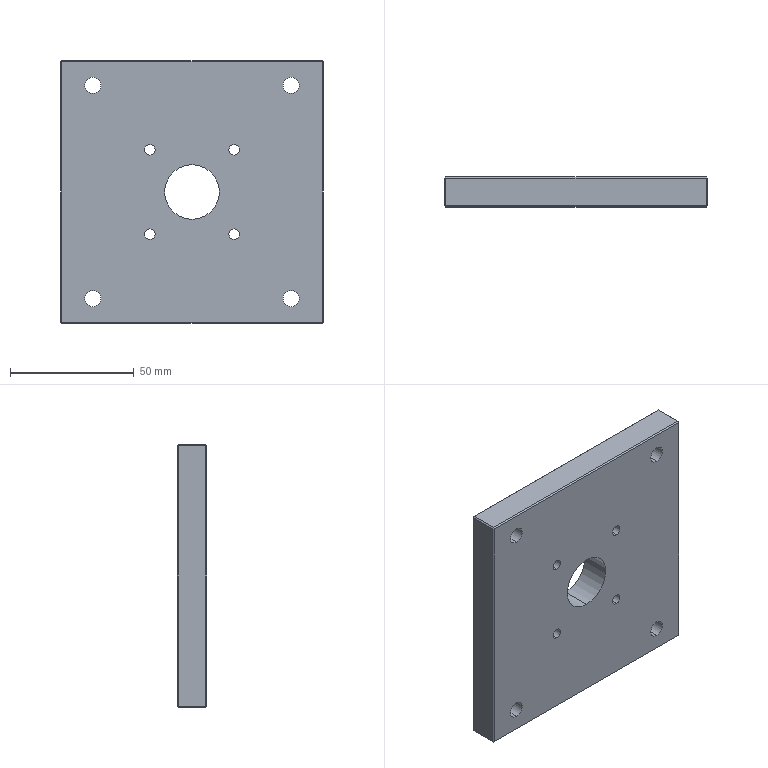Part | STEP file | ND25021-01-JDKM-39-TL | 1 solid | 56 faces | box 106 x 12 x 106 mm | volume 126295 mm3 | plane 30 | cylinder 26 | commonest cylinder face diameters 4.2 x8 6.6 x8 11 x8 22 x2